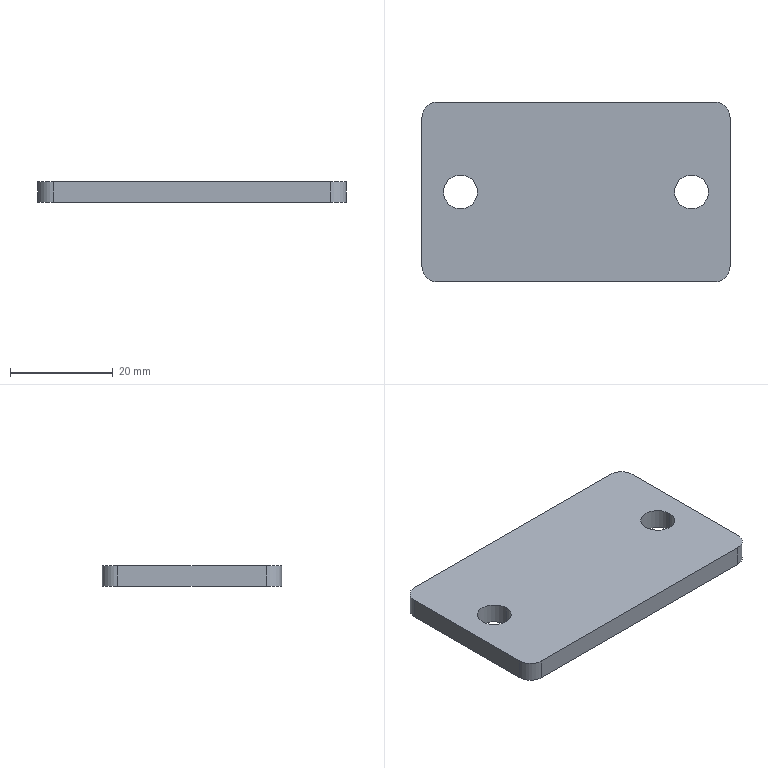Part | SolidWorks | features Extrusion 1, Fillet 1 | 1 solid | 14 faces | box 60 x 35 x 4 mm | volume 8095 mm3 | cylinder 8 | plane 6 | commonest cylinder face diameters 6 x4 6.6 x4
STEP:
#1=CARTESIAN_POINT('',(19.2,0.,4.));
#2=VERTEX_POINT('',#1);
#3=CARTESIAN_POINT('',(25.8,0.,4.));
#4=VERTEX_POINT('',#3);
#5=CARTESIAN_POINT('',(22.5,0.,4.));
#6=DIRECTION('',(0.,0.,1.));
#7=DIRECTION('',(1.,0.,0.));
#8=AXIS2_PLACEMENT_3D('',#5,#6,#7);
#9=CIRCLE('',#8,3.3);
#10=EDGE_CURVE('',#2,#4,#9,.T.);
#11=ORIENTED_EDGE('',*,*,#10,.T.);
#12=CARTESIAN_POINT('',(25.8,0.,0.));
#13=VERTEX_POINT('',#12);
#14=CARTESIAN_POINT('',(25.8,0.,4.));
#15=DIRECTION('',(0.,0.,-1.));
#16=VECTOR('',#15,1000.);
#17=LINE('',#14,#16);
#18=EDGE_CURVE('',#4,#13,#17,.T.);
#19=ORIENTED_EDGE('',*,*,#18,.T.);
#20=CARTESIAN_POINT('',(19.2,0.,0.));
#21=VERTEX_POINT('',#20);
#22=CARTESIAN_POINT('',(22.5,0.,0.));
#23=DIRECTION('',(0.,0.,1.));
#24=DIRECTION('',(1.,0.,0.));
#25=AXIS2_PLACEMENT_3D('',#22,#23,#24);
#26=CIRCLE('',#25,3.3);
#27=EDGE_CURVE('',#21,#13,#26,.T.);
#28=ORIENTED_EDGE('',*,*,#27,.F.);
#29=CARTESIAN_POINT('',(19.2,0.,4.));
#30=DIRECTION('',(0.,0.,-1.));
#31=VECTOR('',#30,1000.);
#32=LINE('',#29,#31);
#33=EDGE_CURVE('',#2,#21,#32,.T.);
#34=ORIENTED_EDGE('',*,*,#33,.F.);
#35=EDGE_LOOP('',(#11,#19,#28,#34));
#36=FACE_OUTER_BOUND('',#35,.T.);
#37=CARTESIAN_POINT('',(22.5,0.,4.));
#38=DIRECTION('',(0.,0.,-1.));
#39=DIRECTION('',(-1.,0.,0.));
#40=AXIS2_PLACEMENT_3D('',#37,#38,#39);
#41=CYLINDRICAL_SURFACE('',#40,3.3);
#42=ADVANCED_FACE('',(#36),#41,.F.);
#43=CARTESIAN_POINT('',(-25.8,0.,4.));
#44=VERTEX_POINT('',#43);
#45=CARTESIAN_POINT('',(-19.2,0.,4.));
#46=VERTEX_POINT('',#45);
#47=CARTESIAN_POINT('',(-22.5,0.,4.));
#48=DIRECTION('',(0.,0.,1.));
#49=DIRECTION('',(1.,0.,0.));
#50=AXIS2_PLACEMENT_3D('',#47,#48,#49);
#51=CIRCLE('',#50,3.3);
#52=EDGE_CURVE('',#44,#46,#51,.T.);
#53=ORIENTED_EDGE('',*,*,#52,.T.);
#54=CARTESIAN_POINT('',(-19.2,0.,0.));
#55=VERTEX_POINT('',#54);
#56=CARTESIAN_POINT('',(-19.2,0.,4.));
#57=DIRECTION('',(0.,0.,-1.));
#58=VECTOR('',#57,1000.);
#59=LINE('',#56,#58);
#60=EDGE_CURVE('',#46,#55,#59,.T.);
#61=ORIENTED_EDGE('',*,*,#60,.T.);
#62=CARTESIAN_POINT('',(-25.8,0.,0.));
#63=VERTEX_POINT('',#62);
#64=CARTESIAN_POINT('',(-22.5,0.,0.));
#65=DIRECTION('',(0.,0.,1.));
#66=DIRECTION('',(1.,0.,0.));
#67=AXIS2_PLACEMENT_3D('',#64,#65,#66);
#68=CIRCLE('',#67,3.3);
#69=EDGE_CURVE('',#63,#55,#68,.T.);
#70=ORIENTED_EDGE('',*,*,#69,.F.);
#71=CARTESIAN_POINT('',(-25.8,0.,4.));
#72=DIRECTION('',(0.,0.,-1.));
#73=VECTOR('',#72,1000.);
#74=LINE('',#71,#73);
#75=EDGE_CURVE('',#44,#63,#74,.T.);
#76=ORIENTED_EDGE('',*,*,#75,.F.);
#77=EDGE_LOOP('',(#53,#61,#70,#76));
#78=FACE_OUTER_BOUND('',#77,.T.);
#79=CARTESIAN_POINT('',(-22.5,0.,4.));
#80=DIRECTION('',(0.,0.,-1.));
#81=DIRECTION('',(-1.,0.,0.));
#82=AXIS2_PLACEMENT_3D('',#79,#80,#81);
#83=CYLINDRICAL_SURFACE('',#82,3.3);
#84=ADVANCED_FACE('',(#78),#83,.F.);
#85=ORIENTED_EDGE('',*,*,#52,.F.);
#86=CARTESIAN_POINT('',(-22.5,0.,4.));
#87=DIRECTION('',(0.,0.,1.));
#88=DIRECTION('',(1.,0.,0.));
#89=AXIS2_PLACEMENT_3D('',#86,#87,#88);
#90=CIRCLE('',#89,3.3);
#91=EDGE_CURVE('',#46,#44,#90,.T.);
#92=ORIENTED_EDGE('',*,*,#91,.F.);
#93=EDGE_LOOP('',(#85,#92));
#94=FACE_BOUND('',#93,.T.);
#95=CARTESIAN_POINT('',(-27.,-17.5,4.));
#96=VERTEX_POINT('',#95);
#97=CARTESIAN_POINT('',(27.,-17.5,4.));
#98=VERTEX_POINT('',#97);
#99=CARTESIAN_POINT('',(-30.,-17.5,4.));
#100=DIRECTION('',(1.,0.,0.));
#101=VECTOR('',#100,1000.);
#102=LINE('',#99,#101);
#103=EDGE_CURVE('',#96,#98,#102,.T.);
#104=ORIENTED_EDGE('',*,*,#103,.T.);
#105=CARTESIAN_POINT('',(30.,-14.5,4.));
#106=VERTEX_POINT('',#105);
#107=CARTESIAN_POINT('',(27.,-14.5,4.));
#108=DIRECTION('',(0.,0.,1.));
#109=DIRECTION('',(1.,0.,0.));
#110=AXIS2_PLACEMENT_3D('',#107,#108,#109);
#111=CIRCLE('',#110,3.);
#112=EDGE_CURVE('',#98,#106,#111,.T.);
#113=ORIENTED_EDGE('',*,*,#112,.T.);
#114=CARTESIAN_POINT('',(30.,14.5,4.));
#115=VERTEX_POINT('',#114);
#116=CARTESIAN_POINT('',(30.,17.5,4.));
#117=DIRECTION('',(0.,1.,0.));
#118=VECTOR('',#117,1000.);
#119=LINE('',#116,#118);
#120=EDGE_CURVE('',#106,#115,#119,.T.);
#121=ORIENTED_EDGE('',*,*,#120,.T.);
#122=CARTESIAN_POINT('',(27.,17.5,4.));
#123=VERTEX_POINT('',#122);
#124=CARTESIAN_POINT('',(27.,14.5,4.));
#125=DIRECTION('',(0.,0.,1.));
#126=DIRECTION('',(1.,0.,0.));
#127=AXIS2_PLACEMENT_3D('',#124,#125,#126);
#128=CIRCLE('',#127,3.);
#129=EDGE_CURVE('',#115,#123,#128,.T.);
#130=ORIENTED_EDGE('',*,*,#129,.T.);
#131=CARTESIAN_POINT('',(-27.,17.5,4.));
#132=VERTEX_POINT('',#131);
#133=CARTESIAN_POINT('',(-30.,17.5,4.));
#134=DIRECTION('',(-1.,0.,0.));
#135=VECTOR('',#134,1000.);
#136=LINE('',#133,#135);
#137=EDGE_CURVE('',#123,#132,#136,.T.);
#138=ORIENTED_EDGE('',*,*,#137,.T.);
#139=CARTESIAN_POINT('',(-30.,14.5,4.));
#140=VERTEX_POINT('',#139);
#141=CARTESIAN_POINT('',(-27.,14.5,4.));
#142=DIRECTION('',(0.,0.,1.));
#143=DIRECTION('',(1.,0.,0.));
#144=AXIS2_PLACEMENT_3D('',#141,#142,#143);
#145=CIRCLE('',#144,3.);
#146=EDGE_CURVE('',#132,#140,#145,.T.);
#147=ORIENTED_EDGE('',*,*,#146,.T.);
#148=CARTESIAN_POINT('',(-30.,-14.5,4.));
#149=VERTEX_POINT('',#148);
#150=CARTESIAN_POINT('',(-30.,17.5,4.));
#151=DIRECTION('',(0.,-1.,0.));
#152=VECTOR('',#151,1000.);
#153=LINE('',#150,#152);
#154=EDGE_CURVE('',#140,#149,#153,.T.);
#155=ORIENTED_EDGE('',*,*,#154,.T.);
#156=CARTESIAN_POINT('',(-27.,-14.5,4.));
#157=DIRECTION('',(0.,0.,1.));
#158=DIRECTION('',(1.,0.,0.));
#159=AXIS2_PLACEMENT_3D('',#156,#157,#158);
#160=CIRCLE('',#159,3.);
#161=EDGE_CURVE('',#149,#96,#160,.T.);
#162=ORIENTED_EDGE('',*,*,#161,.T.);
#163=EDGE_LOOP('',(#104,#113,#121,#130,#138,#147,#155,#162));
#164=FACE_OUTER_BOUND('',#163,.T.);
#165=ORIENTED_EDGE('',*,*,#10,.F.);
#166=CARTESIAN_POINT('',(22.5,0.,4.));
#167=DIRECTION('',(0.,0.,1.));
#168=DIRECTION('',(1.,0.,0.));
#169=AXIS2_PLACEMENT_3D('',#166,#167,#168);
#170=CIRCLE('',#169,3.3);
#171=EDGE_CURVE('',#4,#2,#170,.T.);
#172=ORIENTED_EDGE('',*,*,#171,.F.);
#173=EDGE_LOOP('',(#165,#172));
#174=FACE_BOUND('',#173,.T.);
#175=CARTESIAN_POINT('',(0.,0.,4.));
#176=DIRECTION('',(0.,0.,1.));
#177=DIRECTION('',(1.,0.,0.));
#178=AXIS2_PLACEMENT_3D('',#175,#176,#177);
#179=PLANE('',#178);
#180=ADVANCED_FACE('',(#94,#164,#174),#179,.T.);
#181=CARTESIAN_POINT('',(30.,-14.5,0.));
#182=VERTEX_POINT('',#181);
#183=CARTESIAN_POINT('',(30.,14.5,0.));
#184=VERTEX_POINT('',#183);
#185=CARTESIAN_POINT('',(30.,17.5,0.));
#186=DIRECTION('',(0.,1.,0.));
#187=VECTOR('',#186,1000.);
#188=LINE('',#185,#187);
#189=EDGE_CURVE('',#182,#184,#188,.T.);
#190=ORIENTED_EDGE('',*,*,#189,.F.);
#191=CARTESIAN_POINT('',(27.,-17.5,0.));
#192=VERTEX_POINT('',#191);
#193=CARTESIAN_POINT('',(27.,-14.5,0.));
#194=DIRECTION('',(0.,0.,-1.));
#195=DIRECTION('',(1.,0.,0.));
#196=AXIS2_PLACEMENT_3D('',#193,#194,#195);
#197=CIRCLE('',#196,3.);
#198=EDGE_CURVE('',#182,#192,#197,.T.);
#199=ORIENTED_EDGE('',*,*,#198,.T.);
#200=CARTESIAN_POINT('',(-27.,-17.5,0.));
#201=VERTEX_POINT('',#200);
#202=CARTESIAN_POINT('',(-30.,-17.5,0.));
#203=DIRECTION('',(1.,0.,0.));
#204=VECTOR('',#203,1000.);
#205=LINE('',#202,#204);
#206=EDGE_CURVE('',#201,#192,#205,.T.);
#207=ORIENTED_EDGE('',*,*,#206,.F.);
#208=CARTESIAN_POINT('',(-30.,-14.5,0.));
#209=VERTEX_POINT('',#208);
#210=CARTESIAN_POINT('',(-27.,-14.5,0.));
#211=DIRECTION('',(0.,0.,-1.));
#212=DIRECTION('',(1.,0.,0.));
#213=AXIS2_PLACEMENT_3D('',#210,#211,#212);
#214=CIRCLE('',#213,3.);
#215=EDGE_CURVE('',#201,#209,#214,.T.);
#216=ORIENTED_EDGE('',*,*,#215,.T.);
#217=CARTESIAN_POINT('',(-30.,14.5,0.));
#218=VERTEX_POINT('',#217);
#219=CARTESIAN_POINT('',(-30.,17.5,0.));
#220=DIRECTION('',(0.,-1.,0.));
#221=VECTOR('',#220,1000.);
#222=LINE('',#219,#221);
#223=EDGE_CURVE('',#218,#209,#222,.T.);
#224=ORIENTED_EDGE('',*,*,#223,.F.);
#225=CARTESIAN_POINT('',(-27.,17.5,0.));
#226=VERTEX_POINT('',#225);
#227=CARTESIAN_POINT('',(-27.,14.5,0.));
#228=DIRECTION('',(0.,0.,-1.));
#229=DIRECTION('',(1.,0.,0.));
#230=AXIS2_PLACEMENT_3D('',#227,#228,#229);
#231=CIRCLE('',#230,3.);
#232=EDGE_CURVE('',#218,#226,#231,.T.);
#233=ORIENTED_EDGE('',*,*,#232,.T.);
#234=CARTESIAN_POINT('',(27.,17.5,0.));
#235=VERTEX_POINT('',#234);
#236=CARTESIAN_POINT('',(-30.,17.5,0.));
#237=DIRECTION('',(-1.,0.,0.));
#238=VECTOR('',#237,1000.);
#239=LINE('',#236,#238);
#240=EDGE_CURVE('',#235,#226,#239,.T.);
#241=ORIENTED_EDGE('',*,*,#240,.F.);
#242=CARTESIAN_POINT('',(27.,14.5,0.));
#243=DIRECTION('',(0.,0.,-1.));
#244=DIRECTION('',(1.,0.,0.));
#245=AXIS2_PLACEMENT_3D('',#242,#243,#244);
#246=CIRCLE('',#245,3.);
#247=EDGE_CURVE('',#235,#184,#246,.T.);
#248=ORIENTED_EDGE('',*,*,#247,.T.);
#249=EDGE_LOOP('',(#190,#199,#207,#216,#224,#233,#241,#248));
#250=FACE_OUTER_BOUND('',#249,.T.);
#251=ORIENTED_EDGE('',*,*,#69,.T.);
#252=CARTESIAN_POINT('',(-22.5,0.,0.));
#253=DIRECTION('',(0.,0.,1.));
#254=DIRECTION('',(1.,0.,0.));
#255=AXIS2_PLACEMENT_3D('',#252,#253,#254);
#256=CIRCLE('',#255,3.3);
#257=EDGE_CURVE('',#55,#63,#256,.T.);
#258=ORIENTED_EDGE('',*,*,#257,.T.);
#259=EDGE_LOOP('',(#251,#258));
#260=FACE_BOUND('',#259,.T.);
#261=ORIENTED_EDGE('',*,*,#27,.T.);
#262=CARTESIAN_POINT('',(22.5,0.,0.));
#263=DIRECTION('',(0.,0.,1.));
#264=DIRECTION('',(1.,0.,0.));
#265=AXIS2_PLACEMENT_3D('',#262,#263,#264);
#266=CIRCLE('',#265,3.3);
#267=EDGE_CURVE('',#13,#21,#266,.T.);
#268=ORIENTED_EDGE('',*,*,#267,.T.);
#269=EDGE_LOOP('',(#261,#268));
#270=FACE_BOUND('',#269,.T.);
#271=CARTESIAN_POINT('',(0.,0.,0.));
#272=DIRECTION('',(0.,0.,1.));
#273=DIRECTION('',(1.,0.,0.));
#274=AXIS2_PLACEMENT_3D('',#271,#272,#273);
#275=PLANE('',#274);
#276=ADVANCED_FACE('',(#250,#260,#270),#275,.F.);
#277=ORIENTED_EDGE('',*,*,#120,.F.);
#278=CARTESIAN_POINT('',(30.,-14.5,4.));
#279=DIRECTION('',(0.,0.,-1.));
#280=VECTOR('',#279,1000.);
#281=LINE('',#278,#280);
#282=EDGE_CURVE('',#106,#182,#281,.T.);
#283=ORIENTED_EDGE('',*,*,#282,.T.);
#284=ORIENTED_EDGE('',*,*,#189,.T.);
#285=CARTESIAN_POINT('',(30.,14.5,4.));
#286=DIRECTION('',(0.,0.,1.));
#287=VECTOR('',#286,1000.);
#288=LINE('',#285,#287);
#289=EDGE_CURVE('',#184,#115,#288,.T.);
#290=ORIENTED_EDGE('',*,*,#289,.T.);
#291=EDGE_LOOP('',(#277,#283,#284,#290));
#292=FACE_OUTER_BOUND('',#291,.T.);
#293=CARTESIAN_POINT('',(30.,17.5,4.));
#294=DIRECTION('',(-1.,0.,0.));
#295=DIRECTION('',(0.,-1.,0.));
#296=AXIS2_PLACEMENT_3D('',#293,#294,#295);
#297=PLANE('',#296);
#298=ADVANCED_FACE('',(#292),#297,.F.);
#299=ORIENTED_EDGE('',*,*,#137,.F.);
#300=CARTESIAN_POINT('',(27.,17.5,4.));
#301=DIRECTION('',(0.,0.,-1.));
#302=VECTOR('',#301,1000.);
#303=LINE('',#300,#302);
#304=EDGE_CURVE('',#123,#235,#303,.T.);
#305=ORIENTED_EDGE('',*,*,#304,.T.);
#306=ORIENTED_EDGE('',*,*,#240,.T.);
#307=CARTESIAN_POINT('',(-27.,17.5,4.));
#308=DIRECTION('',(0.,0.,1.));
#309=VECTOR('',#308,1000.);
#310=LINE('',#307,#309);
#311=EDGE_CURVE('',#226,#132,#310,.T.);
#312=ORIENTED_EDGE('',*,*,#311,.T.);
#313=EDGE_LOOP('',(#299,#305,#306,#312));
#314=FACE_OUTER_BOUND('',#313,.T.);
#315=CARTESIAN_POINT('',(-30.,17.5,4.));
#316=DIRECTION('',(0.,-1.,0.));
#317=DIRECTION('',(0.,0.,-1.));
#318=AXIS2_PLACEMENT_3D('',#315,#316,#317);
#319=PLANE('',#318);
#320=ADVANCED_FACE('',(#314),#319,.F.);
#321=ORIENTED_EDGE('',*,*,#223,.T.);
#322=CARTESIAN_POINT('',(-30.,-14.5,4.));
#323=DIRECTION('',(0.,0.,1.));
#324=VECTOR('',#323,1000.);
#325=LINE('',#322,#324);
#326=EDGE_CURVE('',#209,#149,#325,.T.);
#327=ORIENTED_EDGE('',*,*,#326,.T.);
#328=ORIENTED_EDGE('',*,*,#154,.F.);
#329=CARTESIAN_POINT('',(-30.,14.5,4.));
#330=DIRECTION('',(0.,0.,-1.));
#331=VECTOR('',#330,1000.);
#332=LINE('',#329,#331);
#333=EDGE_CURVE('',#140,#218,#332,.T.);
#334=ORIENTED_EDGE('',*,*,#333,.T.);
#335=EDGE_LOOP('',(#321,#327,#328,#334));
#336=FACE_OUTER_BOUND('',#335,.T.);
#337=CARTESIAN_POINT('',(-30.,17.5,4.));
#338=DIRECTION('',(1.,0.,0.));
#339=DIRECTION('',(0.,1.,0.));
#340=AXIS2_PLACEMENT_3D('',#337,#338,#339);
#341=PLANE('',#340);
#342=ADVANCED_FACE('',(#336),#341,.F.);
#343=ORIENTED_EDGE('',*,*,#206,.T.);
#344=CARTESIAN_POINT('',(27.,-17.5,4.));
#345=DIRECTION('',(0.,0.,1.));
#346=VECTOR('',#345,1000.);
#347=LINE('',#344,#346);
#348=EDGE_CURVE('',#192,#98,#347,.T.);
#349=ORIENTED_EDGE('',*,*,#348,.T.);
#350=ORIENTED_EDGE('',*,*,#103,.F.);
#351=CARTESIAN_POINT('',(-27.,-17.5,4.));
#352=DIRECTION('',(0.,0.,-1.));
#353=VECTOR('',#352,1000.);
#354=LINE('',#351,#353);
#355=EDGE_CURVE('',#96,#201,#354,.T.);
#356=ORIENTED_EDGE('',*,*,#355,.T.);
#357=EDGE_LOOP('',(#343,#349,#350,#356));
#358=FACE_OUTER_BOUND('',#357,.T.);
#359=CARTESIAN_POINT('',(-30.,-17.5,4.));
#360=DIRECTION('',(0.,1.,0.));
#361=DIRECTION('',(0.,0.,1.));
#362=AXIS2_PLACEMENT_3D('',#359,#360,#361);
#363=PLANE('',#362);
#364=ADVANCED_FACE('',(#358),#363,.F.);
#365=ORIENTED_EDGE('',*,*,#60,.F.);
#366=ORIENTED_EDGE('',*,*,#91,.T.);
#367=ORIENTED_EDGE('',*,*,#75,.T.);
#368=ORIENTED_EDGE('',*,*,#257,.F.);
#369=EDGE_LOOP('',(#365,#366,#367,#368));
#370=FACE_OUTER_BOUND('',#369,.T.);
#371=CARTESIAN_POINT('',(-22.5,0.,4.));
#372=DIRECTION('',(0.,0.,-1.));
#373=DIRECTION('',(-1.,0.,0.));
#374=AXIS2_PLACEMENT_3D('',#371,#372,#373);
#375=CYLINDRICAL_SURFACE('',#374,3.3);
#376=ADVANCED_FACE('',(#370),#375,.F.);
#377=ORIENTED_EDGE('',*,*,#18,.F.);
#378=ORIENTED_EDGE('',*,*,#171,.T.);
#379=ORIENTED_EDGE('',*,*,#33,.T.);
#380=ORIENTED_EDGE('',*,*,#267,.F.);
#381=EDGE_LOOP('',(#377,#378,#379,#380));
#382=FACE_OUTER_BOUND('',#381,.T.);
#383=CARTESIAN_POINT('',(22.5,0.,4.));
#384=DIRECTION('',(0.,0.,-1.));
#385=DIRECTION('',(-1.,0.,0.));
#386=AXIS2_PLACEMENT_3D('',#383,#384,#385);
#387=CYLINDRICAL_SURFACE('',#386,3.3);
#388=ADVANCED_FACE('',(#382),#387,.F.);
#389=ORIENTED_EDGE('',*,*,#112,.F.);
#390=ORIENTED_EDGE('',*,*,#348,.F.);
#391=ORIENTED_EDGE('',*,*,#198,.F.);
#392=ORIENTED_EDGE('',*,*,#282,.F.);
#393=EDGE_LOOP('',(#389,#390,#391,#392));
#394=FACE_OUTER_BOUND('',#393,.T.);
#395=CARTESIAN_POINT('',(27.,-14.5,4.));
#396=DIRECTION('',(0.,0.,-1.));
#397=DIRECTION('',(-1.,0.,0.));
#398=AXIS2_PLACEMENT_3D('',#395,#396,#397);
#399=CYLINDRICAL_SURFACE('',#398,3.);
#400=ADVANCED_FACE('',(#394),#399,.T.);
#401=ORIENTED_EDGE('',*,*,#129,.F.);
#402=ORIENTED_EDGE('',*,*,#289,.F.);
#403=ORIENTED_EDGE('',*,*,#247,.F.);
#404=ORIENTED_EDGE('',*,*,#304,.F.);
#405=EDGE_LOOP('',(#401,#402,#403,#404));
#406=FACE_OUTER_BOUND('',#405,.T.);
#407=CARTESIAN_POINT('',(27.,14.5,4.));
#408=DIRECTION('',(0.,0.,-1.));
#409=DIRECTION('',(-1.,0.,0.));
#410=AXIS2_PLACEMENT_3D('',#407,#408,#409);
#411=CYLINDRICAL_SURFACE('',#410,3.);
#412=ADVANCED_FACE('',(#406),#411,.T.);
#413=ORIENTED_EDGE('',*,*,#161,.F.);
#414=ORIENTED_EDGE('',*,*,#326,.F.);
#415=ORIENTED_EDGE('',*,*,#215,.F.);
#416=ORIENTED_EDGE('',*,*,#355,.F.);
#417=EDGE_LOOP('',(#413,#414,#415,#416));
#418=FACE_OUTER_BOUND('',#417,.T.);
#419=CARTESIAN_POINT('',(-27.,-14.5,4.));
#420=DIRECTION('',(0.,0.,-1.));
#421=DIRECTION('',(-1.,0.,0.));
#422=AXIS2_PLACEMENT_3D('',#419,#420,#421);
#423=CYLINDRICAL_SURFACE('',#422,3.);
#424=ADVANCED_FACE('',(#418),#423,.T.);
#425=ORIENTED_EDGE('',*,*,#146,.F.);
#426=ORIENTED_EDGE('',*,*,#311,.F.);
#427=ORIENTED_EDGE('',*,*,#232,.F.);
#428=ORIENTED_EDGE('',*,*,#333,.F.);
#429=EDGE_LOOP('',(#425,#426,#427,#428));
#430=FACE_OUTER_BOUND('',#429,.T.);
#431=CARTESIAN_POINT('',(-27.,14.5,4.));
#432=DIRECTION('',(0.,0.,-1.));
#433=DIRECTION('',(-1.,0.,0.));
#434=AXIS2_PLACEMENT_3D('',#431,#432,#433);
#435=CYLINDRICAL_SURFACE('',#434,3.);
#436=ADVANCED_FACE('',(#430),#435,.T.);
#437=CLOSED_SHELL('',(#42,#84,#180,#276,#298,#320,#342,#364,#376,#388,#400,#412,#424,#436));
#438=MANIFOLD_SOLID_BREP('',#437);
#439=CARTESIAN_POINT('',(0.,0.,0.));
#440=DIRECTION('',(0.,0.,1.));
#441=DIRECTION('',(1.,0.,0.));
#442=AXIS2_PLACEMENT_3D('',#439,#440,#441);
#443=(LENGTH_UNIT()NAMED_UNIT(*)SI_UNIT(.MILLI.,.METRE.));
#444=UNCERTAINTY_MEASURE_WITH_UNIT(LENGTH_MEASURE(0.00001),#443,'','');
#445=(NAMED_UNIT(*)PLANE_ANGLE_UNIT()SI_UNIT($,.RADIAN.));
#446=(NAMED_UNIT(*)SI_UNIT($,.STERADIAN.)SOLID_ANGLE_UNIT());
#447=(GEOMETRIC_REPRESENTATION_CONTEXT(3)GLOBAL_UNCERTAINTY_ASSIGNED_CONTEXT((#444))GLOBAL_UNIT_ASSIGNED_CONTEXT((#443,#445,#446))REPRESENTATION_CONTEXT('',''));
#448=ADVANCED_BREP_SHAPE_REPRESENTATION('',(#438,#442),#447);